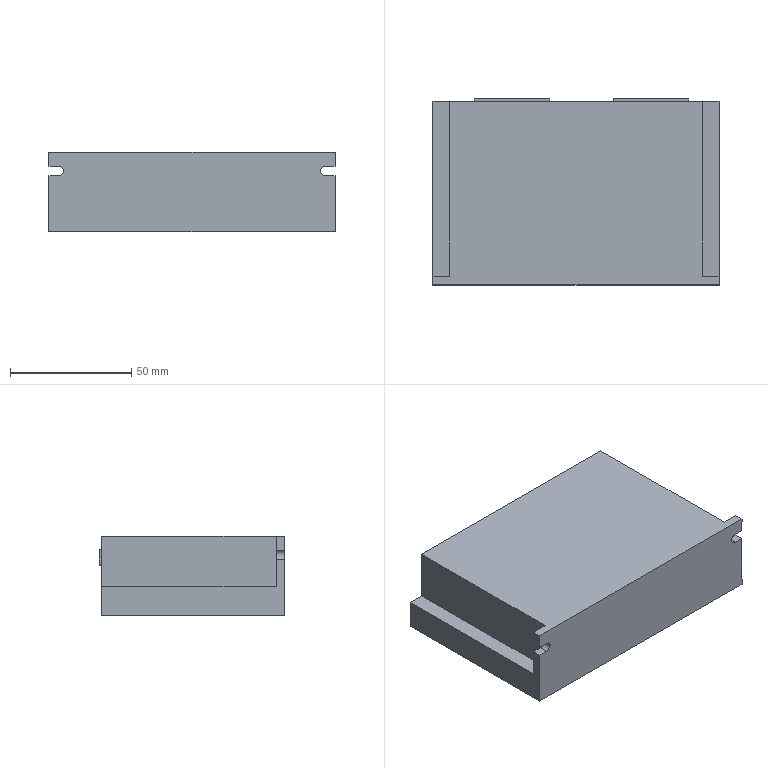Part | NX | features BREP 1 | 1 solid | 35 faces | box 118 x 76.7 x 33 mm | volume 272910 mm3 | plane 33 | cylinder 2 | commonest cylinder face diameters 4 x2
STEP:
#1=CARTESIAN_POINT('',(-41.887,72.7,10.848));
#2=VERTEX_POINT('',#1);
#3=CARTESIAN_POINT('',(-10.887,72.7,10.848));
#4=VERTEX_POINT('',#3);
#5=CARTESIAN_POINT('',(-41.887,72.7,10.848));
#6=DIRECTION('',(1.,0.,0.));
#7=VECTOR('',#6,1000.);
#8=LINE('',#5,#7);
#9=EDGE_CURVE('',#2,#4,#8,.T.);
#10=ORIENTED_EDGE('',*,*,#9,.F.);
#11=CARTESIAN_POINT('',(-41.887,72.7,4.458));
#12=VERTEX_POINT('',#11);
#13=CARTESIAN_POINT('',(-41.887,72.7,4.458));
#14=DIRECTION('',(0.,0.,1.));
#15=VECTOR('',#14,1000.);
#16=LINE('',#13,#15);
#17=EDGE_CURVE('',#12,#2,#16,.T.);
#18=ORIENTED_EDGE('',*,*,#17,.F.);
#19=CARTESIAN_POINT('',(-10.887,72.7,4.458));
#20=VERTEX_POINT('',#19);
#21=CARTESIAN_POINT('',(-41.887,72.7,4.458));
#22=DIRECTION('',(-1.,0.,0.));
#23=VECTOR('',#22,1000.);
#24=LINE('',#21,#23);
#25=EDGE_CURVE('',#20,#12,#24,.T.);
#26=ORIENTED_EDGE('',*,*,#25,.F.);
#27=CARTESIAN_POINT('',(-10.887,72.7,4.458));
#28=DIRECTION('',(0.,0.,-1.));
#29=VECTOR('',#28,1000.);
#30=LINE('',#27,#29);
#31=EDGE_CURVE('',#4,#20,#30,.T.);
#32=ORIENTED_EDGE('',*,*,#31,.F.);
#33=EDGE_LOOP('',(#10,#18,#26,#32));
#34=FACE_BOUND('',#33,.T.);
#35=CARTESIAN_POINT('',(-47.5,72.7,2.5));
#36=VERTEX_POINT('',#35);
#37=CARTESIAN_POINT('',(-47.5,72.7,12.5));
#38=VERTEX_POINT('',#37);
#39=CARTESIAN_POINT('',(-47.5,72.7,2.5));
#40=DIRECTION('',(0.,0.,1.));
#41=VECTOR('',#40,1000.);
#42=LINE('',#39,#41);
#43=EDGE_CURVE('',#36,#38,#42,.T.);
#44=ORIENTED_EDGE('',*,*,#43,.T.);
#45=CARTESIAN_POINT('',(47.5,72.7,12.5));
#46=VERTEX_POINT('',#45);
#47=CARTESIAN_POINT('',(-47.5,72.7,12.5));
#48=DIRECTION('',(1.,0.,0.));
#49=VECTOR('',#48,1000.);
#50=LINE('',#47,#49);
#51=EDGE_CURVE('',#38,#46,#50,.T.);
#52=ORIENTED_EDGE('',*,*,#51,.T.);
#53=CARTESIAN_POINT('',(47.5,72.7,2.5));
#54=VERTEX_POINT('',#53);
#55=CARTESIAN_POINT('',(47.5,72.7,2.5));
#56=DIRECTION('',(0.,0.,-1.));
#57=VECTOR('',#56,1000.);
#58=LINE('',#55,#57);
#59=EDGE_CURVE('',#46,#54,#58,.T.);
#60=ORIENTED_EDGE('',*,*,#59,.T.);
#61=CARTESIAN_POINT('',(-47.5,72.7,2.5));
#62=DIRECTION('',(-1.,0.,0.));
#63=VECTOR('',#62,1000.);
#64=LINE('',#61,#63);
#65=EDGE_CURVE('',#54,#36,#64,.T.);
#66=ORIENTED_EDGE('',*,*,#65,.T.);
#67=EDGE_LOOP('',(#44,#52,#60,#66));
#68=FACE_BOUND('',#67,.T.);
#69=CARTESIAN_POINT('',(15.478,72.7,10.848));
#70=VERTEX_POINT('',#69);
#71=CARTESIAN_POINT('',(46.478,72.7,10.848));
#72=VERTEX_POINT('',#71);
#73=CARTESIAN_POINT('',(15.478,72.7,10.848));
#74=DIRECTION('',(1.,0.,0.));
#75=VECTOR('',#74,1000.);
#76=LINE('',#73,#75);
#77=EDGE_CURVE('',#70,#72,#76,.T.);
#78=ORIENTED_EDGE('',*,*,#77,.F.);
#79=CARTESIAN_POINT('',(15.478,72.7,4.458));
#80=VERTEX_POINT('',#79);
#81=CARTESIAN_POINT('',(15.478,72.7,4.458));
#82=DIRECTION('',(0.,0.,1.));
#83=VECTOR('',#82,1000.);
#84=LINE('',#81,#83);
#85=EDGE_CURVE('',#80,#70,#84,.T.);
#86=ORIENTED_EDGE('',*,*,#85,.F.);
#87=CARTESIAN_POINT('',(46.478,72.7,4.458));
#88=VERTEX_POINT('',#87);
#89=CARTESIAN_POINT('',(15.478,72.7,4.458));
#90=DIRECTION('',(-1.,0.,0.));
#91=VECTOR('',#90,1000.);
#92=LINE('',#89,#91);
#93=EDGE_CURVE('',#88,#80,#92,.T.);
#94=ORIENTED_EDGE('',*,*,#93,.F.);
#95=CARTESIAN_POINT('',(46.478,72.7,4.458));
#96=DIRECTION('',(0.,0.,-1.));
#97=VECTOR('',#96,1000.);
#98=LINE('',#95,#97);
#99=EDGE_CURVE('',#72,#88,#98,.T.);
#100=ORIENTED_EDGE('',*,*,#99,.F.);
#101=EDGE_LOOP('',(#78,#86,#94,#100));
#102=FACE_BOUND('',#101,.T.);
#103=CARTESIAN_POINT('',(0.,72.7,0.));
#104=DIRECTION('',(0.,1.,0.));
#105=DIRECTION('',(0.,0.,1.));
#106=AXIS2_PLACEMENT_3D('',#103,#104,#105);
#107=PLANE('',#106);
#108=ADVANCED_FACE('',(#34,#68,#102),#107,.T.);
#109=CARTESIAN_POINT('',(-59.,3.6,10.7));
#110=VERTEX_POINT('',#109);
#111=CARTESIAN_POINT('',(-59.,3.6,16.5));
#112=VERTEX_POINT('',#111);
#113=CARTESIAN_POINT('',(-59.,3.6,16.5));
#114=DIRECTION('',(0.,0.,1.));
#115=VECTOR('',#114,1000.);
#116=LINE('',#113,#115);
#117=EDGE_CURVE('',#110,#112,#116,.T.);
#118=ORIENTED_EDGE('',*,*,#117,.F.);
#119=CARTESIAN_POINT('',(-59.,0.,10.7));
#120=VERTEX_POINT('',#119);
#121=CARTESIAN_POINT('',(-59.,75.7,10.7));
#122=DIRECTION('',(0.,-1.,0.));
#123=VECTOR('',#122,1000.);
#124=LINE('',#121,#123);
#125=EDGE_CURVE('',#110,#120,#124,.T.);
#126=ORIENTED_EDGE('',*,*,#125,.T.);
#127=CARTESIAN_POINT('',(-59.,0.,16.5));
#128=VERTEX_POINT('',#127);
#129=CARTESIAN_POINT('',(-59.,0.,-16.5));
#130=DIRECTION('',(0.,0.,1.));
#131=VECTOR('',#130,1000.);
#132=LINE('',#129,#131);
#133=EDGE_CURVE('',#120,#128,#132,.T.);
#134=ORIENTED_EDGE('',*,*,#133,.T.);
#135=CARTESIAN_POINT('',(-59.,75.7,16.5));
#136=DIRECTION('',(0.,-1.,0.));
#137=VECTOR('',#136,1000.);
#138=LINE('',#135,#137);
#139=EDGE_CURVE('',#112,#128,#138,.T.);
#140=ORIENTED_EDGE('',*,*,#139,.F.);
#141=EDGE_LOOP('',(#118,#126,#134,#140));
#142=FACE_BOUND('',#141,.T.);
#143=CARTESIAN_POINT('',(-59.,75.7,-16.5));
#144=DIRECTION('',(1.,0.,0.));
#145=DIRECTION('',(0.,0.,-1.));
#146=AXIS2_PLACEMENT_3D('',#143,#144,#145);
#147=PLANE('',#146);
#148=ADVANCED_FACE('',(#142),#147,.F.);
#149=CARTESIAN_POINT('',(59.,3.6,6.7));
#150=VERTEX_POINT('',#149);
#151=CARTESIAN_POINT('',(59.,3.6,-4.5));
#152=VERTEX_POINT('',#151);
#153=CARTESIAN_POINT('',(59.,3.6,16.5));
#154=DIRECTION('',(0.,0.,-1.));
#155=VECTOR('',#154,1000.);
#156=LINE('',#153,#155);
#157=EDGE_CURVE('',#150,#152,#156,.T.);
#158=ORIENTED_EDGE('',*,*,#157,.F.);
#159=CARTESIAN_POINT('',(59.,0.,6.7));
#160=VERTEX_POINT('',#159);
#161=CARTESIAN_POINT('',(59.,75.7,6.7));
#162=DIRECTION('',(0.,-1.,0.));
#163=VECTOR('',#162,1000.);
#164=LINE('',#161,#163);
#165=EDGE_CURVE('',#150,#160,#164,.T.);
#166=ORIENTED_EDGE('',*,*,#165,.T.);
#167=CARTESIAN_POINT('',(59.,0.,-16.5));
#168=VERTEX_POINT('',#167);
#169=CARTESIAN_POINT('',(59.,0.,-16.5));
#170=DIRECTION('',(0.,0.,-1.));
#171=VECTOR('',#170,1000.);
#172=LINE('',#169,#171);
#173=EDGE_CURVE('',#160,#168,#172,.T.);
#174=ORIENTED_EDGE('',*,*,#173,.T.);
#175=CARTESIAN_POINT('',(59.,75.7,-16.5));
#176=VERTEX_POINT('',#175);
#177=CARTESIAN_POINT('',(59.,75.7,-16.5));
#178=DIRECTION('',(0.,-1.,0.));
#179=VECTOR('',#178,1000.);
#180=LINE('',#177,#179);
#181=EDGE_CURVE('',#176,#168,#180,.T.);
#182=ORIENTED_EDGE('',*,*,#181,.F.);
#183=CARTESIAN_POINT('',(59.,75.7,-4.5));
#184=VERTEX_POINT('',#183);
#185=CARTESIAN_POINT('',(59.,75.7,-16.5));
#186=DIRECTION('',(0.,0.,-1.));
#187=VECTOR('',#186,1000.);
#188=LINE('',#185,#187);
#189=EDGE_CURVE('',#184,#176,#188,.T.);
#190=ORIENTED_EDGE('',*,*,#189,.F.);
#191=CARTESIAN_POINT('',(59.,3.6,-4.5));
#192=DIRECTION('',(0.,1.,0.));
#193=VECTOR('',#192,1000.);
#194=LINE('',#191,#193);
#195=EDGE_CURVE('',#152,#184,#194,.T.);
#196=ORIENTED_EDGE('',*,*,#195,.F.);
#197=EDGE_LOOP('',(#158,#166,#174,#182,#190,#196));
#198=FACE_BOUND('',#197,.T.);
#199=CARTESIAN_POINT('',(59.,75.7,-16.5));
#200=DIRECTION('',(-1.,0.,0.));
#201=DIRECTION('',(0.,0.,1.));
#202=AXIS2_PLACEMENT_3D('',#199,#200,#201);
#203=PLANE('',#202);
#204=ADVANCED_FACE('',(#198),#203,.F.);
#205=CARTESIAN_POINT('',(59.,0.,16.5));
#206=VERTEX_POINT('',#205);
#207=CARTESIAN_POINT('',(59.,0.,10.7));
#208=VERTEX_POINT('',#207);
#209=CARTESIAN_POINT('',(59.,0.,-16.5));
#210=DIRECTION('',(0.,0.,-1.));
#211=VECTOR('',#210,1000.);
#212=LINE('',#209,#211);
#213=EDGE_CURVE('',#206,#208,#212,.T.);
#214=ORIENTED_EDGE('',*,*,#213,.T.);
#215=CARTESIAN_POINT('',(59.,3.6,10.7));
#216=VERTEX_POINT('',#215);
#217=CARTESIAN_POINT('',(59.,75.7,10.7));
#218=DIRECTION('',(0.,1.,0.));
#219=VECTOR('',#218,1000.);
#220=LINE('',#217,#219);
#221=EDGE_CURVE('',#208,#216,#220,.T.);
#222=ORIENTED_EDGE('',*,*,#221,.T.);
#223=CARTESIAN_POINT('',(59.,3.6,16.5));
#224=VERTEX_POINT('',#223);
#225=CARTESIAN_POINT('',(59.,3.6,16.5));
#226=DIRECTION('',(0.,0.,-1.));
#227=VECTOR('',#226,1000.);
#228=LINE('',#225,#227);
#229=EDGE_CURVE('',#224,#216,#228,.T.);
#230=ORIENTED_EDGE('',*,*,#229,.F.);
#231=CARTESIAN_POINT('',(59.,75.7,16.5));
#232=DIRECTION('',(0.,-1.,0.));
#233=VECTOR('',#232,1000.);
#234=LINE('',#231,#233);
#235=EDGE_CURVE('',#224,#206,#234,.T.);
#236=ORIENTED_EDGE('',*,*,#235,.T.);
#237=EDGE_LOOP('',(#214,#222,#230,#236));
#238=FACE_BOUND('',#237,.T.);
#239=CARTESIAN_POINT('',(59.,75.7,-16.5));
#240=DIRECTION('',(-1.,0.,0.));
#241=DIRECTION('',(0.,0.,1.));
#242=AXIS2_PLACEMENT_3D('',#239,#240,#241);
#243=PLANE('',#242);
#244=ADVANCED_FACE('',(#238),#243,.F.);
#245=CARTESIAN_POINT('',(-59.,0.,-16.5));
#246=VERTEX_POINT('',#245);
#247=CARTESIAN_POINT('',(-59.,0.,-16.5));
#248=DIRECTION('',(-1.,0.,0.));
#249=VECTOR('',#248,1000.);
#250=LINE('',#247,#249);
#251=EDGE_CURVE('',#168,#246,#250,.T.);
#252=ORIENTED_EDGE('',*,*,#251,.T.);
#253=CARTESIAN_POINT('',(-59.,75.7,-16.5));
#254=VERTEX_POINT('',#253);
#255=CARTESIAN_POINT('',(-59.,75.7,-16.5));
#256=DIRECTION('',(0.,-1.,0.));
#257=VECTOR('',#256,1000.);
#258=LINE('',#255,#257);
#259=EDGE_CURVE('',#254,#246,#258,.T.);
#260=ORIENTED_EDGE('',*,*,#259,.F.);
#261=CARTESIAN_POINT('',(-59.,75.7,-16.5));
#262=DIRECTION('',(-1.,0.,0.));
#263=VECTOR('',#262,1000.);
#264=LINE('',#261,#263);
#265=EDGE_CURVE('',#176,#254,#264,.T.);
#266=ORIENTED_EDGE('',*,*,#265,.F.);
#267=ORIENTED_EDGE('',*,*,#181,.T.);
#268=EDGE_LOOP('',(#252,#260,#266,#267));
#269=FACE_BOUND('',#268,.T.);
#270=CARTESIAN_POINT('',(-59.,75.7,-16.5));
#271=DIRECTION('',(0.,0.,1.));
#272=DIRECTION('',(1.,0.,0.));
#273=AXIS2_PLACEMENT_3D('',#270,#271,#272);
#274=PLANE('',#273);
#275=ADVANCED_FACE('',(#269),#274,.F.);
#276=CARTESIAN_POINT('',(-59.,0.,6.7));
#277=VERTEX_POINT('',#276);
#278=CARTESIAN_POINT('',(-59.,0.,-16.5));
#279=DIRECTION('',(0.,0.,1.));
#280=VECTOR('',#279,1000.);
#281=LINE('',#278,#280);
#282=EDGE_CURVE('',#246,#277,#281,.T.);
#283=ORIENTED_EDGE('',*,*,#282,.T.);
#284=CARTESIAN_POINT('',(-59.,3.6,6.7));
#285=VERTEX_POINT('',#284);
#286=CARTESIAN_POINT('',(-59.,75.7,6.7));
#287=DIRECTION('',(0.,1.,0.));
#288=VECTOR('',#287,1000.);
#289=LINE('',#286,#288);
#290=EDGE_CURVE('',#277,#285,#289,.T.);
#291=ORIENTED_EDGE('',*,*,#290,.T.);
#292=CARTESIAN_POINT('',(-59.,3.6,-4.5));
#293=VERTEX_POINT('',#292);
#294=CARTESIAN_POINT('',(-59.,3.6,16.5));
#295=DIRECTION('',(0.,0.,1.));
#296=VECTOR('',#295,1000.);
#297=LINE('',#294,#296);
#298=EDGE_CURVE('',#293,#285,#297,.T.);
#299=ORIENTED_EDGE('',*,*,#298,.F.);
#300=CARTESIAN_POINT('',(-59.,75.7,-4.5));
#301=VERTEX_POINT('',#300);
#302=CARTESIAN_POINT('',(-59.,3.6,-4.5));
#303=DIRECTION('',(0.,1.,0.));
#304=VECTOR('',#303,1000.);
#305=LINE('',#302,#304);
#306=EDGE_CURVE('',#293,#301,#305,.T.);
#307=ORIENTED_EDGE('',*,*,#306,.T.);
#308=CARTESIAN_POINT('',(-59.,75.7,-16.5));
#309=DIRECTION('',(0.,0.,1.));
#310=VECTOR('',#309,1000.);
#311=LINE('',#308,#310);
#312=EDGE_CURVE('',#254,#301,#311,.T.);
#313=ORIENTED_EDGE('',*,*,#312,.F.);
#314=ORIENTED_EDGE('',*,*,#259,.T.);
#315=EDGE_LOOP('',(#283,#291,#299,#307,#313,#314));
#316=FACE_BOUND('',#315,.T.);
#317=CARTESIAN_POINT('',(-59.,75.7,-16.5));
#318=DIRECTION('',(1.,0.,0.));
#319=DIRECTION('',(0.,0.,-1.));
#320=AXIS2_PLACEMENT_3D('',#317,#318,#319);
#321=PLANE('',#320);
#322=ADVANCED_FACE('',(#316),#321,.F.);
#323=CARTESIAN_POINT('',(-52.25,75.7,16.5));
#324=VERTEX_POINT('',#323);
#325=CARTESIAN_POINT('',(52.25,75.7,16.5));
#326=VERTEX_POINT('',#325);
#327=CARTESIAN_POINT('',(-59.,75.7,16.5));
#328=DIRECTION('',(1.,0.,0.));
#329=VECTOR('',#328,1000.);
#330=LINE('',#327,#329);
#331=EDGE_CURVE('',#324,#326,#330,.T.);
#332=ORIENTED_EDGE('',*,*,#331,.F.);
#333=CARTESIAN_POINT('',(-52.25,3.6,16.5));
#334=VERTEX_POINT('',#333);
#335=CARTESIAN_POINT('',(-52.25,3.6,16.5));
#336=DIRECTION('',(0.,1.,0.));
#337=VECTOR('',#336,1000.);
#338=LINE('',#335,#337);
#339=EDGE_CURVE('',#334,#324,#338,.T.);
#340=ORIENTED_EDGE('',*,*,#339,.F.);
#341=CARTESIAN_POINT('',(-59.,3.6,16.5));
#342=DIRECTION('',(1.,0.,0.));
#343=VECTOR('',#342,1000.);
#344=LINE('',#341,#343);
#345=EDGE_CURVE('',#112,#334,#344,.T.);
#346=ORIENTED_EDGE('',*,*,#345,.F.);
#347=ORIENTED_EDGE('',*,*,#139,.T.);
#348=CARTESIAN_POINT('',(-59.,0.,16.5));
#349=DIRECTION('',(1.,0.,0.));
#350=VECTOR('',#349,1000.);
#351=LINE('',#348,#350);
#352=EDGE_CURVE('',#128,#206,#351,.T.);
#353=ORIENTED_EDGE('',*,*,#352,.T.);
#354=ORIENTED_EDGE('',*,*,#235,.F.);
#355=CARTESIAN_POINT('',(52.25,3.6,16.5));
#356=VERTEX_POINT('',#355);
#357=CARTESIAN_POINT('',(59.,3.6,16.5));
#358=DIRECTION('',(1.,0.,0.));
#359=VECTOR('',#358,1000.);
#360=LINE('',#357,#359);
#361=EDGE_CURVE('',#356,#224,#360,.T.);
#362=ORIENTED_EDGE('',*,*,#361,.F.);
#363=CARTESIAN_POINT('',(52.25,3.6,16.5));
#364=DIRECTION('',(0.,1.,0.));
#365=VECTOR('',#364,1000.);
#366=LINE('',#363,#365);
#367=EDGE_CURVE('',#356,#326,#366,.T.);
#368=ORIENTED_EDGE('',*,*,#367,.T.);
#369=EDGE_LOOP('',(#332,#340,#346,#347,#353,#354,#362,#368));
#370=FACE_BOUND('',#369,.T.);
#371=CARTESIAN_POINT('',(-59.,75.7,16.5));
#372=DIRECTION('',(0.,0.,-1.));
#373=DIRECTION('',(-1.,0.,0.));
#374=AXIS2_PLACEMENT_3D('',#371,#372,#373);
#375=PLANE('',#374);
#376=ADVANCED_FACE('',(#370),#375,.F.);
#377=CARTESIAN_POINT('',(-47.5,75.7,2.5));
#378=VERTEX_POINT('',#377);
#379=CARTESIAN_POINT('',(-47.5,75.7,12.5));
#380=VERTEX_POINT('',#379);
#381=CARTESIAN_POINT('',(-47.5,75.7,2.5));
#382=DIRECTION('',(0.,0.,1.));
#383=VECTOR('',#382,1000.);
#384=LINE('',#381,#383);
#385=EDGE_CURVE('',#378,#380,#384,.T.);
#386=ORIENTED_EDGE('',*,*,#385,.F.);
#387=CARTESIAN_POINT('',(47.5,75.7,2.5));
#388=VERTEX_POINT('',#387);
#389=CARTESIAN_POINT('',(-47.5,75.7,2.5));
#390=DIRECTION('',(-1.,0.,0.));
#391=VECTOR('',#390,1000.);
#392=LINE('',#389,#391);
#393=EDGE_CURVE('',#388,#378,#392,.T.);
#394=ORIENTED_EDGE('',*,*,#393,.F.);
#395=CARTESIAN_POINT('',(47.5,75.7,12.5));
#396=VERTEX_POINT('',#395);
#397=CARTESIAN_POINT('',(47.5,75.7,2.5));
#398=DIRECTION('',(0.,0.,-1.));
#399=VECTOR('',#398,1000.);
#400=LINE('',#397,#399);
#401=EDGE_CURVE('',#396,#388,#400,.T.);
#402=ORIENTED_EDGE('',*,*,#401,.F.);
#403=CARTESIAN_POINT('',(-47.5,75.7,12.5));
#404=DIRECTION('',(1.,0.,0.));
#405=VECTOR('',#404,1000.);
#406=LINE('',#403,#405);
#407=EDGE_CURVE('',#380,#396,#406,.T.);
#408=ORIENTED_EDGE('',*,*,#407,.F.);
#409=EDGE_LOOP('',(#386,#394,#402,#408));
#410=FACE_BOUND('',#409,.T.);
#411=CARTESIAN_POINT('',(-52.25,75.7,-4.5));
#412=VERTEX_POINT('',#411);
#413=CARTESIAN_POINT('',(-59.,75.7,-4.5));
#414=DIRECTION('',(-1.,0.,0.));
#415=VECTOR('',#414,1000.);
#416=LINE('',#413,#415);
#417=EDGE_CURVE('',#412,#301,#416,.T.);
#418=ORIENTED_EDGE('',*,*,#417,.F.);
#419=CARTESIAN_POINT('',(-52.25,75.7,16.5));
#420=DIRECTION('',(0.,0.,-1.));
#421=VECTOR('',#420,1000.);
#422=LINE('',#419,#421);
#423=EDGE_CURVE('',#324,#412,#422,.T.);
#424=ORIENTED_EDGE('',*,*,#423,.F.);
#425=ORIENTED_EDGE('',*,*,#331,.T.);
#426=CARTESIAN_POINT('',(52.25,75.7,-4.5));
#427=VERTEX_POINT('',#426);
#428=CARTESIAN_POINT('',(52.25,75.7,16.5));
#429=DIRECTION('',(0.,0.,1.));
#430=VECTOR('',#429,1000.);
#431=LINE('',#428,#430);
#432=EDGE_CURVE('',#427,#326,#431,.T.);
#433=ORIENTED_EDGE('',*,*,#432,.F.);
#434=CARTESIAN_POINT('',(59.,75.7,-4.5));
#435=DIRECTION('',(-1.,0.,0.));
#436=VECTOR('',#435,1000.);
#437=LINE('',#434,#436);
#438=EDGE_CURVE('',#184,#427,#437,.T.);
#439=ORIENTED_EDGE('',*,*,#438,.F.);
#440=ORIENTED_EDGE('',*,*,#189,.T.);
#441=ORIENTED_EDGE('',*,*,#265,.T.);
#442=ORIENTED_EDGE('',*,*,#312,.T.);
#443=EDGE_LOOP('',(#418,#424,#425,#433,#439,#440,#441,#442));
#444=FACE_BOUND('',#443,.T.);
#445=CARTESIAN_POINT('',(0.,75.7,0.));
#446=DIRECTION('',(0.,1.,0.));
#447=DIRECTION('',(0.,0.,1.));
#448=AXIS2_PLACEMENT_3D('',#445,#446,#447);
#449=PLANE('',#448);
#450=ADVANCED_FACE('',(#410,#444),#449,.T.);
#451=ORIENTED_EDGE('',*,*,#133,.F.);
#452=CARTESIAN_POINT('',(-55.,0.,10.7));
#453=VERTEX_POINT('',#452);
#454=CARTESIAN_POINT('',(0.,0.,10.7));
#455=DIRECTION('',(1.,0.,0.));
#456=VECTOR('',#455,1000.);
#457=LINE('',#454,#456);
#458=EDGE_CURVE('',#120,#453,#457,.T.);
#459=ORIENTED_EDGE('',*,*,#458,.T.);
#460=CARTESIAN_POINT('',(-55.,0.,6.7));
#461=VERTEX_POINT('',#460);
#462=CARTESIAN_POINT('',(-55.,0.,8.7));
#463=DIRECTION('',(0.,1.,0.));
#464=DIRECTION('',(0.,0.,1.));
#465=AXIS2_PLACEMENT_3D('',#462,#463,#464);
#466=CIRCLE('',#465,2.);
#467=EDGE_CURVE('',#453,#461,#466,.T.);
#468=ORIENTED_EDGE('',*,*,#467,.T.);
#469=CARTESIAN_POINT('',(0.,0.,6.7));
#470=DIRECTION('',(-1.,0.,0.));
#471=VECTOR('',#470,1000.);
#472=LINE('',#469,#471);
#473=EDGE_CURVE('',#461,#277,#472,.T.);
#474=ORIENTED_EDGE('',*,*,#473,.T.);
#475=ORIENTED_EDGE('',*,*,#282,.F.);
#476=ORIENTED_EDGE('',*,*,#251,.F.);
#477=ORIENTED_EDGE('',*,*,#173,.F.);
#478=CARTESIAN_POINT('',(55.,0.,6.7));
#479=VERTEX_POINT('',#478);
#480=CARTESIAN_POINT('',(0.,0.,6.7));
#481=DIRECTION('',(-1.,0.,0.));
#482=VECTOR('',#481,1000.);
#483=LINE('',#480,#482);
#484=EDGE_CURVE('',#160,#479,#483,.T.);
#485=ORIENTED_EDGE('',*,*,#484,.T.);
#486=CARTESIAN_POINT('',(55.,0.,10.7));
#487=VERTEX_POINT('',#486);
#488=CARTESIAN_POINT('',(55.,0.,8.7));
#489=DIRECTION('',(0.,1.,0.));
#490=DIRECTION('',(0.,0.,1.));
#491=AXIS2_PLACEMENT_3D('',#488,#489,#490);
#492=CIRCLE('',#491,2.);
#493=EDGE_CURVE('',#479,#487,#492,.T.);
#494=ORIENTED_EDGE('',*,*,#493,.T.);
#495=CARTESIAN_POINT('',(0.,0.,10.7));
#496=DIRECTION('',(1.,0.,0.));
#497=VECTOR('',#496,1000.);
#498=LINE('',#495,#497);
#499=EDGE_CURVE('',#487,#208,#498,.T.);
#500=ORIENTED_EDGE('',*,*,#499,.T.);
#501=ORIENTED_EDGE('',*,*,#213,.F.);
#502=ORIENTED_EDGE('',*,*,#352,.F.);
#503=EDGE_LOOP('',(#451,#459,#468,#474,#475,#476,#477,#485,#494,#500,#501,#502));
#504=FACE_BOUND('',#503,.T.);
#505=CARTESIAN_POINT('',(0.,0.,0.));
#506=DIRECTION('',(0.,1.,0.));
#507=DIRECTION('',(0.,0.,1.));
#508=AXIS2_PLACEMENT_3D('',#505,#506,#507);
#509=PLANE('',#508);
#510=ADVANCED_FACE('',(#504),#509,.F.);
#511=ORIENTED_EDGE('',*,*,#432,.T.);
#512=ORIENTED_EDGE('',*,*,#367,.F.);
#513=CARTESIAN_POINT('',(52.25,3.6,-4.5));
#514=VERTEX_POINT('',#513);
#515=CARTESIAN_POINT('',(52.25,3.6,16.5));
#516=DIRECTION('',(0.,0.,1.));
#517=VECTOR('',#516,1000.);
#518=LINE('',#515,#517);
#519=EDGE_CURVE('',#514,#356,#518,.T.);
#520=ORIENTED_EDGE('',*,*,#519,.F.);
#521=CARTESIAN_POINT('',(52.25,3.6,-4.5));
#522=DIRECTION('',(0.,1.,0.));
#523=VECTOR('',#522,1000.);
#524=LINE('',#521,#523);
#525=EDGE_CURVE('',#514,#427,#524,.T.);
#526=ORIENTED_EDGE('',*,*,#525,.T.);
#527=EDGE_LOOP('',(#511,#512,#520,#526));
#528=FACE_BOUND('',#527,.T.);
#529=CARTESIAN_POINT('',(52.25,3.6,16.5));
#530=DIRECTION('',(-1.,0.,0.));
#531=DIRECTION('',(0.,0.,1.));
#532=AXIS2_PLACEMENT_3D('',#529,#530,#531);
#533=PLANE('',#532);
#534=ADVANCED_FACE('',(#528),#533,.F.);
#535=ORIENTED_EDGE('',*,*,#438,.T.);
#536=ORIENTED_EDGE('',*,*,#525,.F.);
#537=CARTESIAN_POINT('',(59.,3.6,-4.5));
#538=DIRECTION('',(-1.,0.,0.));
#539=VECTOR('',#538,1000.);
#540=LINE('',#537,#539);
#541=EDGE_CURVE('',#152,#514,#540,.T.);
#542=ORIENTED_EDGE('',*,*,#541,.F.);
#543=ORIENTED_EDGE('',*,*,#195,.T.);
#544=EDGE_LOOP('',(#535,#536,#542,#543));
#545=FACE_BOUND('',#544,.T.);
#546=CARTESIAN_POINT('',(59.,3.6,-4.5));
#547=DIRECTION('',(0.,0.,-1.));
#548=DIRECTION('',(-1.,0.,0.));
#549=AXIS2_PLACEMENT_3D('',#546,#547,#548);
#550=PLANE('',#549);
#551=ADVANCED_FACE('',(#545),#550,.F.);
#552=CARTESIAN_POINT('',(55.,3.6,6.7));
#553=VERTEX_POINT('',#552);
#554=CARTESIAN_POINT('',(0.,3.6,6.7));
#555=DIRECTION('',(-1.,0.,0.));
#556=VECTOR('',#555,1000.);
#557=LINE('',#554,#556);
#558=EDGE_CURVE('',#150,#553,#557,.T.);
#559=ORIENTED_EDGE('',*,*,#558,.F.);
#560=ORIENTED_EDGE('',*,*,#157,.T.);
#561=ORIENTED_EDGE('',*,*,#541,.T.);
#562=ORIENTED_EDGE('',*,*,#519,.T.);
#563=ORIENTED_EDGE('',*,*,#361,.T.);
#564=ORIENTED_EDGE('',*,*,#229,.T.);
#565=CARTESIAN_POINT('',(55.,3.6,10.7));
#566=VERTEX_POINT('',#565);
#567=CARTESIAN_POINT('',(55.,3.6,10.7));
#568=DIRECTION('',(1.,0.,0.));
#569=VECTOR('',#568,1000.);
#570=LINE('',#567,#569);
#571=EDGE_CURVE('',#566,#216,#570,.T.);
#572=ORIENTED_EDGE('',*,*,#571,.F.);
#573=CARTESIAN_POINT('',(55.,3.6,8.7));
#574=DIRECTION('',(0.,1.,0.));
#575=DIRECTION('',(0.,0.,1.));
#576=AXIS2_PLACEMENT_3D('',#573,#574,#575);
#577=CIRCLE('',#576,2.);
#578=EDGE_CURVE('',#553,#566,#577,.T.);
#579=ORIENTED_EDGE('',*,*,#578,.F.);
#580=EDGE_LOOP('',(#559,#560,#561,#562,#563,#564,#572,#579));
#581=FACE_BOUND('',#580,.T.);
#582=CARTESIAN_POINT('',(0.,3.6,0.));
#583=DIRECTION('',(0.,1.,0.));
#584=DIRECTION('',(0.,0.,1.));
#585=AXIS2_PLACEMENT_3D('',#582,#583,#584);
#586=PLANE('',#585);
#587=ADVANCED_FACE('',(#581),#586,.T.);
#588=ORIENTED_EDGE('',*,*,#417,.T.);
#589=ORIENTED_EDGE('',*,*,#306,.F.);
#590=CARTESIAN_POINT('',(-52.25,3.6,-4.5));
#591=VERTEX_POINT('',#590);
#592=CARTESIAN_POINT('',(-59.,3.6,-4.5));
#593=DIRECTION('',(-1.,0.,0.));
#594=VECTOR('',#593,1000.);
#595=LINE('',#592,#594);
#596=EDGE_CURVE('',#591,#293,#595,.T.);
#597=ORIENTED_EDGE('',*,*,#596,.F.);
#598=CARTESIAN_POINT('',(-52.25,3.6,-4.5));
#599=DIRECTION('',(0.,1.,0.));
#600=VECTOR('',#599,1000.);
#601=LINE('',#598,#600);
#602=EDGE_CURVE('',#591,#412,#601,.T.);
#603=ORIENTED_EDGE('',*,*,#602,.T.);
#604=EDGE_LOOP('',(#588,#589,#597,#603));
#605=FACE_BOUND('',#604,.T.);
#606=CARTESIAN_POINT('',(-59.,3.6,-4.5));
#607=DIRECTION('',(0.,0.,-1.));
#608=DIRECTION('',(-1.,0.,0.));
#609=AXIS2_PLACEMENT_3D('',#606,#607,#608);
#610=PLANE('',#609);
#611=ADVANCED_FACE('',(#605),#610,.F.);
#612=ORIENTED_EDGE('',*,*,#423,.T.);
#613=ORIENTED_EDGE('',*,*,#602,.F.);
#614=CARTESIAN_POINT('',(-52.25,3.6,16.5));
#615=DIRECTION('',(0.,0.,-1.));
#616=VECTOR('',#615,1000.);
#617=LINE('',#614,#616);
#618=EDGE_CURVE('',#334,#591,#617,.T.);
#619=ORIENTED_EDGE('',*,*,#618,.F.);
#620=ORIENTED_EDGE('',*,*,#339,.T.);
#621=EDGE_LOOP('',(#612,#613,#619,#620));
#622=FACE_BOUND('',#621,.T.);
#623=CARTESIAN_POINT('',(-52.25,3.6,16.5));
#624=DIRECTION('',(1.,0.,0.));
#625=DIRECTION('',(0.,0.,-1.));
#626=AXIS2_PLACEMENT_3D('',#623,#624,#625);
#627=PLANE('',#626);
#628=ADVANCED_FACE('',(#622),#627,.F.);
#629=CARTESIAN_POINT('',(-55.,3.6,10.7));
#630=VERTEX_POINT('',#629);
#631=CARTESIAN_POINT('',(0.,3.6,10.7));
#632=DIRECTION('',(1.,0.,0.));
#633=VECTOR('',#632,1000.);
#634=LINE('',#631,#633);
#635=EDGE_CURVE('',#110,#630,#634,.T.);
#636=ORIENTED_EDGE('',*,*,#635,.F.);
#637=ORIENTED_EDGE('',*,*,#117,.T.);
#638=ORIENTED_EDGE('',*,*,#345,.T.);
#639=ORIENTED_EDGE('',*,*,#618,.T.);
#640=ORIENTED_EDGE('',*,*,#596,.T.);
#641=ORIENTED_EDGE('',*,*,#298,.T.);
#642=CARTESIAN_POINT('',(-55.,3.6,6.7));
#643=VERTEX_POINT('',#642);
#644=CARTESIAN_POINT('',(-55.,3.6,6.7));
#645=DIRECTION('',(-1.,0.,0.));
#646=VECTOR('',#645,1000.);
#647=LINE('',#644,#646);
#648=EDGE_CURVE('',#643,#285,#647,.T.);
#649=ORIENTED_EDGE('',*,*,#648,.F.);
#650=CARTESIAN_POINT('',(-55.,3.6,8.7));
#651=DIRECTION('',(0.,1.,0.));
#652=DIRECTION('',(0.,0.,-1.));
#653=AXIS2_PLACEMENT_3D('',#650,#651,#652);
#654=CIRCLE('',#653,2.);
#655=EDGE_CURVE('',#630,#643,#654,.T.);
#656=ORIENTED_EDGE('',*,*,#655,.F.);
#657=EDGE_LOOP('',(#636,#637,#638,#639,#640,#641,#649,#656));
#658=FACE_BOUND('',#657,.T.);
#659=CARTESIAN_POINT('',(0.,3.6,0.));
#660=DIRECTION('',(0.,1.,0.));
#661=DIRECTION('',(0.,0.,1.));
#662=AXIS2_PLACEMENT_3D('',#659,#660,#661);
#663=PLANE('',#662);
#664=ADVANCED_FACE('',(#658),#663,.T.);
#665=CARTESIAN_POINT('',(55.,-68.5,6.7));
#666=DIRECTION('',(0.,1.,0.));
#667=VECTOR('',#666,1000.);
#668=LINE('',#665,#667);
#669=EDGE_CURVE('',#479,#553,#668,.T.);
#670=ORIENTED_EDGE('',*,*,#669,.T.);
#671=ORIENTED_EDGE('',*,*,#578,.T.);
#672=CARTESIAN_POINT('',(55.,-68.5,10.7));
#673=DIRECTION('',(0.,1.,0.));
#674=VECTOR('',#673,1000.);
#675=LINE('',#672,#674);
#676=EDGE_CURVE('',#487,#566,#675,.T.);
#677=ORIENTED_EDGE('',*,*,#676,.F.);
#678=ORIENTED_EDGE('',*,*,#493,.F.);
#679=EDGE_LOOP('',(#670,#671,#677,#678));
#680=FACE_BOUND('',#679,.T.);
#681=CARTESIAN_POINT('',(55.,-68.5,8.7));
#682=DIRECTION('',(0.,1.,0.));
#683=DIRECTION('',(0.,0.,1.));
#684=AXIS2_PLACEMENT_3D('',#681,#682,#683);
#685=CYLINDRICAL_SURFACE('',#684,2.);
#686=ADVANCED_FACE('',(#680),#685,.F.);
#687=ORIENTED_EDGE('',*,*,#558,.T.);
#688=ORIENTED_EDGE('',*,*,#669,.F.);
#689=ORIENTED_EDGE('',*,*,#484,.F.);
#690=ORIENTED_EDGE('',*,*,#165,.F.);
#691=EDGE_LOOP('',(#687,#688,#689,#690));
#692=FACE_BOUND('',#691,.T.);
#693=CARTESIAN_POINT('',(55.,-68.5,6.7));
#694=DIRECTION('',(0.,0.,-1.));
#695=DIRECTION('',(-1.,0.,0.));
#696=AXIS2_PLACEMENT_3D('',#693,#694,#695);
#697=PLANE('',#696);
#698=ADVANCED_FACE('',(#692),#697,.F.);
#699=ORIENTED_EDGE('',*,*,#499,.F.);
#700=ORIENTED_EDGE('',*,*,#676,.T.);
#701=ORIENTED_EDGE('',*,*,#571,.T.);
#702=ORIENTED_EDGE('',*,*,#221,.F.);
#703=EDGE_LOOP('',(#699,#700,#701,#702));
#704=FACE_BOUND('',#703,.T.);
#705=CARTESIAN_POINT('',(55.,-68.5,10.7));
#706=DIRECTION('',(0.,0.,1.));
#707=DIRECTION('',(1.,0.,0.));
#708=AXIS2_PLACEMENT_3D('',#705,#706,#707);
#709=PLANE('',#708);
#710=ADVANCED_FACE('',(#704),#709,.F.);
#711=CARTESIAN_POINT('',(-55.,-68.5,10.7));
#712=DIRECTION('',(0.,1.,0.));
#713=VECTOR('',#712,1000.);
#714=LINE('',#711,#713);
#715=EDGE_CURVE('',#453,#630,#714,.T.);
#716=ORIENTED_EDGE('',*,*,#715,.T.);
#717=ORIENTED_EDGE('',*,*,#655,.T.);
#718=CARTESIAN_POINT('',(-55.,-68.5,6.7));
#719=DIRECTION('',(0.,1.,0.));
#720=VECTOR('',#719,1000.);
#721=LINE('',#718,#720);
#722=EDGE_CURVE('',#461,#643,#721,.T.);
#723=ORIENTED_EDGE('',*,*,#722,.F.);
#724=ORIENTED_EDGE('',*,*,#467,.F.);
#725=EDGE_LOOP('',(#716,#717,#723,#724));
#726=FACE_BOUND('',#725,.T.);
#727=CARTESIAN_POINT('',(-55.,-68.5,8.7));
#728=DIRECTION('',(0.,1.,0.));
#729=DIRECTION('',(0.,0.,1.));
#730=AXIS2_PLACEMENT_3D('',#727,#728,#729);
#731=CYLINDRICAL_SURFACE('',#730,2.);
#732=ADVANCED_FACE('',(#726),#731,.F.);
#733=ORIENTED_EDGE('',*,*,#635,.T.);
#734=ORIENTED_EDGE('',*,*,#715,.F.);
#735=ORIENTED_EDGE('',*,*,#458,.F.);
#736=ORIENTED_EDGE('',*,*,#125,.F.);
#737=EDGE_LOOP('',(#733,#734,#735,#736));
#738=FACE_BOUND('',#737,.T.);
#739=CARTESIAN_POINT('',(-55.,-68.5,10.7));
#740=DIRECTION('',(0.,0.,1.));
#741=DIRECTION('',(1.,0.,0.));
#742=AXIS2_PLACEMENT_3D('',#739,#740,#741);
#743=PLANE('',#742);
#744=ADVANCED_FACE('',(#738),#743,.F.);
#745=ORIENTED_EDGE('',*,*,#473,.F.);
#746=ORIENTED_EDGE('',*,*,#722,.T.);
#747=ORIENTED_EDGE('',*,*,#648,.T.);
#748=ORIENTED_EDGE('',*,*,#290,.F.);
#749=EDGE_LOOP('',(#745,#746,#747,#748));
#750=FACE_BOUND('',#749,.T.);
#751=CARTESIAN_POINT('',(-55.,-68.5,6.7));
#752=DIRECTION('',(0.,0.,-1.));
#753=DIRECTION('',(-1.,0.,0.));
#754=AXIS2_PLACEMENT_3D('',#751,#752,#753);
#755=PLANE('',#754);
#756=ADVANCED_FACE('',(#750),#755,.F.);
#757=ORIENTED_EDGE('',*,*,#385,.T.);
#758=CARTESIAN_POINT('',(-47.5,72.7,12.5));
#759=DIRECTION('',(0.,1.,0.));
#760=VECTOR('',#759,1000.);
#761=LINE('',#758,#760);
#762=EDGE_CURVE('',#38,#380,#761,.T.);
#763=ORIENTED_EDGE('',*,*,#762,.F.);
#764=ORIENTED_EDGE('',*,*,#43,.F.);
#765=CARTESIAN_POINT('',(-47.5,72.7,2.5));
#766=DIRECTION('',(0.,1.,0.));
#767=VECTOR('',#766,1000.);
#768=LINE('',#765,#767);
#769=EDGE_CURVE('',#36,#378,#768,.T.);
#770=ORIENTED_EDGE('',*,*,#769,.T.);
#771=EDGE_LOOP('',(#757,#763,#764,#770));
#772=FACE_BOUND('',#771,.T.);
#773=CARTESIAN_POINT('',(-47.5,72.7,2.5));
#774=DIRECTION('',(-1.,0.,0.));
#775=DIRECTION('',(0.,0.,1.));
#776=AXIS2_PLACEMENT_3D('',#773,#774,#775);
#777=PLANE('',#776);
#778=ADVANCED_FACE('',(#772),#777,.F.);
#779=ORIENTED_EDGE('',*,*,#393,.T.);
#780=ORIENTED_EDGE('',*,*,#769,.F.);
#781=ORIENTED_EDGE('',*,*,#65,.F.);
#782=CARTESIAN_POINT('',(47.5,72.7,2.5));
#783=DIRECTION('',(0.,1.,0.));
#784=VECTOR('',#783,1000.);
#785=LINE('',#782,#784);
#786=EDGE_CURVE('',#54,#388,#785,.T.);
#787=ORIENTED_EDGE('',*,*,#786,.T.);
#788=EDGE_LOOP('',(#779,#780,#781,#787));
#789=FACE_BOUND('',#788,.T.);
#790=CARTESIAN_POINT('',(-47.5,72.7,2.5));
#791=DIRECTION('',(0.,0.,-1.));
#792=DIRECTION('',(-1.,0.,0.));
#793=AXIS2_PLACEMENT_3D('',#790,#791,#792);
#794=PLANE('',#793);
#795=ADVANCED_FACE('',(#789),#794,.F.);
#796=ORIENTED_EDGE('',*,*,#401,.T.);
#797=ORIENTED_EDGE('',*,*,#786,.F.);
#798=ORIENTED_EDGE('',*,*,#59,.F.);
#799=CARTESIAN_POINT('',(47.5,72.7,12.5));
#800=DIRECTION('',(0.,1.,0.));
#801=VECTOR('',#800,1000.);
#802=LINE('',#799,#801);
#803=EDGE_CURVE('',#46,#396,#802,.T.);
#804=ORIENTED_EDGE('',*,*,#803,.T.);
#805=EDGE_LOOP('',(#796,#797,#798,#804));
#806=FACE_BOUND('',#805,.T.);
#807=CARTESIAN_POINT('',(47.5,72.7,2.5));
#808=DIRECTION('',(1.,0.,0.));
#809=DIRECTION('',(0.,0.,-1.));
#810=AXIS2_PLACEMENT_3D('',#807,#808,#809);
#811=PLANE('',#810);
#812=ADVANCED_FACE('',(#806),#811,.F.);
#813=ORIENTED_EDGE('',*,*,#407,.T.);
#814=ORIENTED_EDGE('',*,*,#803,.F.);
#815=ORIENTED_EDGE('',*,*,#51,.F.);
#816=ORIENTED_EDGE('',*,*,#762,.T.);
#817=EDGE_LOOP('',(#813,#814,#815,#816));
#818=FACE_BOUND('',#817,.T.);
#819=CARTESIAN_POINT('',(-47.5,72.7,12.5));
#820=DIRECTION('',(0.,0.,1.));
#821=DIRECTION('',(1.,0.,0.));
#822=AXIS2_PLACEMENT_3D('',#819,#820,#821);
#823=PLANE('',#822);
#824=ADVANCED_FACE('',(#818),#823,.F.);
#825=ORIENTED_EDGE('',*,*,#17,.T.);
#826=CARTESIAN_POINT('',(-41.887,76.7,10.848));
#827=VERTEX_POINT('',#826);
#828=CARTESIAN_POINT('',(-41.887,76.7,10.848));
#829=DIRECTION('',(0.,-1.,0.));
#830=VECTOR('',#829,1000.);
#831=LINE('',#828,#830);
#832=EDGE_CURVE('',#827,#2,#831,.T.);
#833=ORIENTED_EDGE('',*,*,#832,.F.);
#834=CARTESIAN_POINT('',(-41.887,76.7,4.458));
#835=VERTEX_POINT('',#834);
#836=CARTESIAN_POINT('',(-41.887,76.7,4.458));
#837=DIRECTION('',(0.,0.,1.));
#838=VECTOR('',#837,1000.);
#839=LINE('',#836,#838);
#840=EDGE_CURVE('',#835,#827,#839,.T.);
#841=ORIENTED_EDGE('',*,*,#840,.F.);
#842=CARTESIAN_POINT('',(-41.887,76.7,4.458));
#843=DIRECTION('',(0.,-1.,0.));
#844=VECTOR('',#843,1000.);
#845=LINE('',#842,#844);
#846=EDGE_CURVE('',#835,#12,#845,.T.);
#847=ORIENTED_EDGE('',*,*,#846,.T.);
#848=EDGE_LOOP('',(#825,#833,#841,#847));
#849=FACE_BOUND('',#848,.T.);
#850=CARTESIAN_POINT('',(-41.887,76.7,4.458));
#851=DIRECTION('',(1.,0.,0.));
#852=DIRECTION('',(0.,0.,-1.));
#853=AXIS2_PLACEMENT_3D('',#850,#851,#852);
#854=PLANE('',#853);
#855=ADVANCED_FACE('',(#849),#854,.F.);
#856=ORIENTED_EDGE('',*,*,#9,.T.);
#857=CARTESIAN_POINT('',(-10.887,76.7,10.848));
#858=VERTEX_POINT('',#857);
#859=CARTESIAN_POINT('',(-10.887,76.7,10.848));
#860=DIRECTION('',(0.,-1.,0.));
#861=VECTOR('',#860,1000.);
#862=LINE('',#859,#861);
#863=EDGE_CURVE('',#858,#4,#862,.T.);
#864=ORIENTED_EDGE('',*,*,#863,.F.);
#865=CARTESIAN_POINT('',(-41.887,76.7,10.848));
#866=DIRECTION('',(1.,0.,0.));
#867=VECTOR('',#866,1000.);
#868=LINE('',#865,#867);
#869=EDGE_CURVE('',#827,#858,#868,.T.);
#870=ORIENTED_EDGE('',*,*,#869,.F.);
#871=ORIENTED_EDGE('',*,*,#832,.T.);
#872=EDGE_LOOP('',(#856,#864,#870,#871));
#873=FACE_BOUND('',#872,.T.);
#874=CARTESIAN_POINT('',(-41.887,76.7,10.848));
#875=DIRECTION('',(0.,0.,-1.));
#876=DIRECTION('',(-1.,0.,0.));
#877=AXIS2_PLACEMENT_3D('',#874,#875,#876);
#878=PLANE('',#877);
#879=ADVANCED_FACE('',(#873),#878,.F.);
#880=ORIENTED_EDGE('',*,*,#31,.T.);
#881=CARTESIAN_POINT('',(-10.887,76.7,4.458));
#882=VERTEX_POINT('',#881);
#883=CARTESIAN_POINT('',(-10.887,76.7,4.458));
#884=DIRECTION('',(0.,-1.,0.));
#885=VECTOR('',#884,1000.);
#886=LINE('',#883,#885);
#887=EDGE_CURVE('',#882,#20,#886,.T.);
#888=ORIENTED_EDGE('',*,*,#887,.F.);
#889=CARTESIAN_POINT('',(-10.887,76.7,4.458));
#890=DIRECTION('',(0.,0.,-1.));
#891=VECTOR('',#890,1000.);
#892=LINE('',#889,#891);
#893=EDGE_CURVE('',#858,#882,#892,.T.);
#894=ORIENTED_EDGE('',*,*,#893,.F.);
#895=ORIENTED_EDGE('',*,*,#863,.T.);
#896=EDGE_LOOP('',(#880,#888,#894,#895));
#897=FACE_BOUND('',#896,.T.);
#898=CARTESIAN_POINT('',(-10.887,76.7,4.458));
#899=DIRECTION('',(-1.,0.,0.));
#900=DIRECTION('',(0.,0.,1.));
#901=AXIS2_PLACEMENT_3D('',#898,#899,#900);
#902=PLANE('',#901);
#903=ADVANCED_FACE('',(#897),#902,.F.);
#904=ORIENTED_EDGE('',*,*,#25,.T.);
#905=ORIENTED_EDGE('',*,*,#846,.F.);
#906=CARTESIAN_POINT('',(-41.887,76.7,4.458));
#907=DIRECTION('',(-1.,0.,0.));
#908=VECTOR('',#907,1000.);
#909=LINE('',#906,#908);
#910=EDGE_CURVE('',#882,#835,#909,.T.);
#911=ORIENTED_EDGE('',*,*,#910,.F.);
#912=ORIENTED_EDGE('',*,*,#887,.T.);
#913=EDGE_LOOP('',(#904,#905,#911,#912));
#914=FACE_BOUND('',#913,.T.);
#915=CARTESIAN_POINT('',(-41.887,76.7,4.458));
#916=DIRECTION('',(0.,0.,1.));
#917=DIRECTION('',(1.,0.,0.));
#918=AXIS2_PLACEMENT_3D('',#915,#916,#917);
#919=PLANE('',#918);
#920=ADVANCED_FACE('',(#914),#919,.F.);
#921=ORIENTED_EDGE('',*,*,#840,.T.);
#922=ORIENTED_EDGE('',*,*,#869,.T.);
#923=ORIENTED_EDGE('',*,*,#893,.T.);
#924=ORIENTED_EDGE('',*,*,#910,.T.);
#925=EDGE_LOOP('',(#921,#922,#923,#924));
#926=FACE_BOUND('',#925,.T.);
#927=CARTESIAN_POINT('',(0.,76.7,0.));
#928=DIRECTION('',(0.,1.,0.));
#929=DIRECTION('',(0.,0.,1.));
#930=AXIS2_PLACEMENT_3D('',#927,#928,#929);
#931=PLANE('',#930);
#932=ADVANCED_FACE('',(#926),#931,.T.);
#933=ORIENTED_EDGE('',*,*,#85,.T.);
#934=CARTESIAN_POINT('',(15.478,76.7,10.848));
#935=VERTEX_POINT('',#934);
#936=CARTESIAN_POINT('',(15.478,76.7,10.848));
#937=DIRECTION('',(0.,-1.,0.));
#938=VECTOR('',#937,1000.);
#939=LINE('',#936,#938);
#940=EDGE_CURVE('',#935,#70,#939,.T.);
#941=ORIENTED_EDGE('',*,*,#940,.F.);
#942=CARTESIAN_POINT('',(15.478,76.7,4.458));
#943=VERTEX_POINT('',#942);
#944=CARTESIAN_POINT('',(15.478,76.7,4.458));
#945=DIRECTION('',(0.,0.,1.));
#946=VECTOR('',#945,1000.);
#947=LINE('',#944,#946);
#948=EDGE_CURVE('',#943,#935,#947,.T.);
#949=ORIENTED_EDGE('',*,*,#948,.F.);
#950=CARTESIAN_POINT('',(15.478,76.7,4.458));
#951=DIRECTION('',(0.,-1.,0.));
#952=VECTOR('',#951,1000.);
#953=LINE('',#950,#952);
#954=EDGE_CURVE('',#943,#80,#953,.T.);
#955=ORIENTED_EDGE('',*,*,#954,.T.);
#956=EDGE_LOOP('',(#933,#941,#949,#955));
#957=FACE_BOUND('',#956,.T.);
#958=CARTESIAN_POINT('',(15.478,76.7,4.458));
#959=DIRECTION('',(1.,0.,0.));
#960=DIRECTION('',(0.,0.,-1.));
#961=AXIS2_PLACEMENT_3D('',#958,#959,#960);
#962=PLANE('',#961);
#963=ADVANCED_FACE('',(#957),#962,.F.);
#964=ORIENTED_EDGE('',*,*,#77,.T.);
#965=CARTESIAN_POINT('',(46.478,76.7,10.848));
#966=VERTEX_POINT('',#965);
#967=CARTESIAN_POINT('',(46.478,76.7,10.848));
#968=DIRECTION('',(0.,-1.,0.));
#969=VECTOR('',#968,1000.);
#970=LINE('',#967,#969);
#971=EDGE_CURVE('',#966,#72,#970,.T.);
#972=ORIENTED_EDGE('',*,*,#971,.F.);
#973=CARTESIAN_POINT('',(15.478,76.7,10.848));
#974=DIRECTION('',(1.,0.,0.));
#975=VECTOR('',#974,1000.);
#976=LINE('',#973,#975);
#977=EDGE_CURVE('',#935,#966,#976,.T.);
#978=ORIENTED_EDGE('',*,*,#977,.F.);
#979=ORIENTED_EDGE('',*,*,#940,.T.);
#980=EDGE_LOOP('',(#964,#972,#978,#979));
#981=FACE_BOUND('',#980,.T.);
#982=CARTESIAN_POINT('',(15.478,76.7,10.848));
#983=DIRECTION('',(0.,0.,-1.));
#984=DIRECTION('',(-1.,0.,0.));
#985=AXIS2_PLACEMENT_3D('',#982,#983,#984);
#986=PLANE('',#985);
#987=ADVANCED_FACE('',(#981),#986,.F.);
#988=ORIENTED_EDGE('',*,*,#99,.T.);
#989=CARTESIAN_POINT('',(46.478,76.7,4.458));
#990=VERTEX_POINT('',#989);
#991=CARTESIAN_POINT('',(46.478,76.7,4.458));
#992=DIRECTION('',(0.,-1.,0.));
#993=VECTOR('',#992,1000.);
#994=LINE('',#991,#993);
#995=EDGE_CURVE('',#990,#88,#994,.T.);
#996=ORIENTED_EDGE('',*,*,#995,.F.);
#997=CARTESIAN_POINT('',(46.478,76.7,4.458));
#998=DIRECTION('',(0.,0.,-1.));
#999=VECTOR('',#998,1000.);
#1000=LINE('',#997,#999);
#1001=EDGE_CURVE('',#966,#990,#1000,.T.);
#1002=ORIENTED_EDGE('',*,*,#1001,.F.);
#1003=ORIENTED_EDGE('',*,*,#971,.T.);
#1004=EDGE_LOOP('',(#988,#996,#1002,#1003));
#1005=FACE_BOUND('',#1004,.T.);
#1006=CARTESIAN_POINT('',(46.478,76.7,4.458));
#1007=DIRECTION('',(-1.,0.,0.));
#1008=DIRECTION('',(0.,0.,1.));
#1009=AXIS2_PLACEMENT_3D('',#1006,#1007,#1008);
#1010=PLANE('',#1009);
#1011=ADVANCED_FACE('',(#1005),#1010,.F.);
#1012=ORIENTED_EDGE('',*,*,#93,.T.);
#1013=ORIENTED_EDGE('',*,*,#954,.F.);
#1014=CARTESIAN_POINT('',(15.478,76.7,4.458));
#1015=DIRECTION('',(-1.,0.,0.));
#1016=VECTOR('',#1015,1000.);
#1017=LINE('',#1014,#1016);
#1018=EDGE_CURVE('',#990,#943,#1017,.T.);
#1019=ORIENTED_EDGE('',*,*,#1018,.F.);
#1020=ORIENTED_EDGE('',*,*,#995,.T.);
#1021=EDGE_LOOP('',(#1012,#1013,#1019,#1020));
#1022=FACE_BOUND('',#1021,.T.);
#1023=CARTESIAN_POINT('',(15.478,76.7,4.458));
#1024=DIRECTION('',(0.,0.,1.));
#1025=DIRECTION('',(1.,0.,0.));
#1026=AXIS2_PLACEMENT_3D('',#1023,#1024,#1025);
#1027=PLANE('',#1026);
#1028=ADVANCED_FACE('',(#1022),#1027,.F.);
#1029=ORIENTED_EDGE('',*,*,#948,.T.);
#1030=ORIENTED_EDGE('',*,*,#977,.T.);
#1031=ORIENTED_EDGE('',*,*,#1001,.T.);
#1032=ORIENTED_EDGE('',*,*,#1018,.T.);
#1033=EDGE_LOOP('',(#1029,#1030,#1031,#1032));
#1034=FACE_BOUND('',#1033,.T.);
#1035=CARTESIAN_POINT('',(0.,76.7,0.));
#1036=DIRECTION('',(0.,1.,0.));
#1037=DIRECTION('',(0.,0.,1.));
#1038=AXIS2_PLACEMENT_3D('',#1035,#1036,#1037);
#1039=PLANE('',#1038);
#1040=ADVANCED_FACE('',(#1034),#1039,.T.);
#1041=CLOSED_SHELL('',(#108,#148,#204,#244,#275,#322,#376,#450,#510,#534,#551,#587,#611,#628,#664,#686,#698,#710,#732,#744,#756,#778,#795,#812,#824,#855,#879,#903,#920,#932,#963,#987,#1011,#1028,#1040));
#1042=MANIFOLD_SOLID_BREP('',#1041);
#1043=(LENGTH_UNIT()NAMED_UNIT(*)SI_UNIT(.MILLI.,.METRE.));
#1044=UNCERTAINTY_MEASURE_WITH_UNIT(LENGTH_MEASURE(0.00001),#1043,'','');
#1045=(NAMED_UNIT(*)PLANE_ANGLE_UNIT()SI_UNIT($,.RADIAN.));
#1046=(NAMED_UNIT(*)SI_UNIT($,.STERADIAN.)SOLID_ANGLE_UNIT());
#1047=(GEOMETRIC_REPRESENTATION_CONTEXT(3)GLOBAL_UNCERTAINTY_ASSIGNED_CONTEXT((#1044))GLOBAL_UNIT_ASSIGNED_CONTEXT((#1043,#1045,#1046))REPRESENTATION_CONTEXT('',''));
#1048=ADVANCED_BREP_SHAPE_REPRESENTATION('',(#1042),#1047);